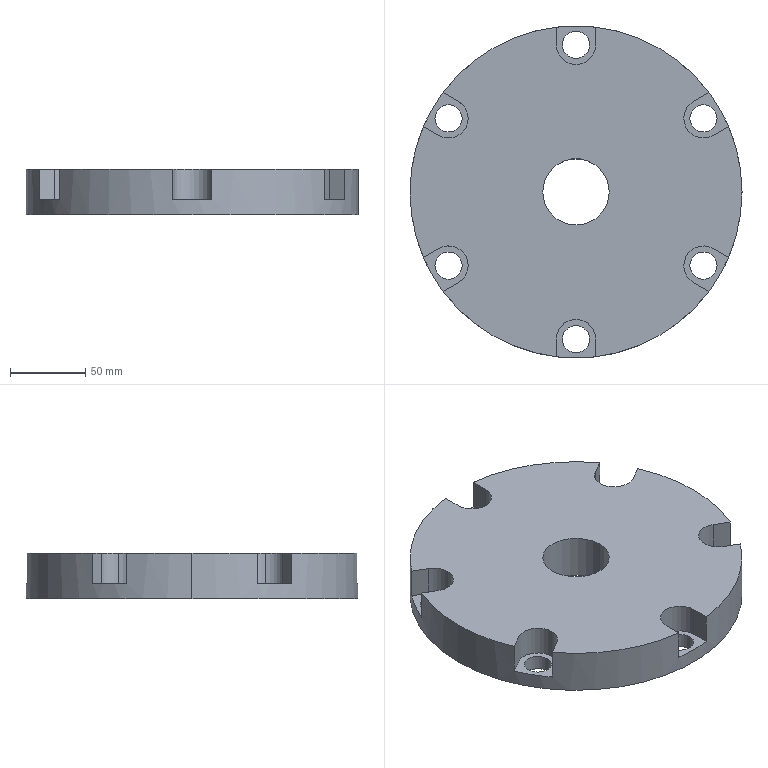Part | SolidWorks | features Extrusion 1, ICE 1 | 1 solid | 44 faces | box 220 x 220 x 30 mm | volume 1009459 mm3 | cylinder 24 | plane 20 | commonest cylinder face diameters 18 x12 26 x8 44 x2 220 x2
STEP:
#1=CARTESIAN_POINT('',(-71.437,-48.75,10.));
#2=VERTEX_POINT('',#1);
#3=CARTESIAN_POINT('',(-90.937,-37.492,10.));
#4=VERTEX_POINT('',#3);
#5=CARTESIAN_POINT('',(-84.437,-48.75,10.));
#6=DIRECTION('',(0.,0.,1.));
#7=DIRECTION('',(1.,0.,0.));
#8=AXIS2_PLACEMENT_3D('',#5,#6,#7);
#9=CIRCLE('',#8,13.);
#10=EDGE_CURVE('',#2,#4,#9,.T.);
#11=ORIENTED_EDGE('',*,*,#10,.F.);
#12=CARTESIAN_POINT('',(-71.437,-48.75,30.));
#13=VERTEX_POINT('',#12);
#14=CARTESIAN_POINT('',(-71.437,-48.75,10.));
#15=DIRECTION('',(0.,0.,1.));
#16=VECTOR('',#15,1000.);
#17=LINE('',#14,#16);
#18=EDGE_CURVE('',#2,#13,#17,.T.);
#19=ORIENTED_EDGE('',*,*,#18,.T.);
#20=CARTESIAN_POINT('',(-90.937,-37.492,30.));
#21=VERTEX_POINT('',#20);
#22=CARTESIAN_POINT('',(-84.437,-48.75,30.));
#23=DIRECTION('',(0.,0.,1.));
#24=DIRECTION('',(1.,0.,0.));
#25=AXIS2_PLACEMENT_3D('',#22,#23,#24);
#26=CIRCLE('',#25,13.);
#27=EDGE_CURVE('',#13,#21,#26,.T.);
#28=ORIENTED_EDGE('',*,*,#27,.T.);
#29=CARTESIAN_POINT('',(-90.937,-37.492,10.));
#30=DIRECTION('',(0.,0.,1.));
#31=VECTOR('',#30,1000.);
#32=LINE('',#29,#31);
#33=EDGE_CURVE('',#4,#21,#32,.T.);
#34=ORIENTED_EDGE('',*,*,#33,.F.);
#35=EDGE_LOOP('',(#11,#19,#28,#34));
#36=FACE_OUTER_BOUND('',#35,.T.);
#37=CARTESIAN_POINT('',(-84.437,-48.75,10.));
#38=DIRECTION('',(0.,0.,1.));
#39=DIRECTION('',(1.,0.,0.));
#40=AXIS2_PLACEMENT_3D('',#37,#38,#39);
#41=CYLINDRICAL_SURFACE('',#40,13.);
#42=ADVANCED_FACE('',(#36),#41,.F.);
#43=CARTESIAN_POINT('',(-71.437,48.75,10.));
#44=VERTEX_POINT('',#43);
#45=CARTESIAN_POINT('',(-77.937,60.008,10.));
#46=VERTEX_POINT('',#45);
#47=CARTESIAN_POINT('',(-84.437,48.75,10.));
#48=DIRECTION('',(0.,0.,1.));
#49=DIRECTION('',(1.,0.,0.));
#50=AXIS2_PLACEMENT_3D('',#47,#48,#49);
#51=CIRCLE('',#50,13.);
#52=EDGE_CURVE('',#44,#46,#51,.T.);
#53=ORIENTED_EDGE('',*,*,#52,.F.);
#54=CARTESIAN_POINT('',(-71.437,48.75,30.));
#55=VERTEX_POINT('',#54);
#56=CARTESIAN_POINT('',(-71.437,48.75,10.));
#57=DIRECTION('',(0.,0.,1.));
#58=VECTOR('',#57,1000.);
#59=LINE('',#56,#58);
#60=EDGE_CURVE('',#44,#55,#59,.T.);
#61=ORIENTED_EDGE('',*,*,#60,.T.);
#62=CARTESIAN_POINT('',(-77.937,60.008,30.));
#63=VERTEX_POINT('',#62);
#64=CARTESIAN_POINT('',(-84.437,48.75,30.));
#65=DIRECTION('',(0.,0.,1.));
#66=DIRECTION('',(1.,0.,0.));
#67=AXIS2_PLACEMENT_3D('',#64,#65,#66);
#68=CIRCLE('',#67,13.);
#69=EDGE_CURVE('',#55,#63,#68,.T.);
#70=ORIENTED_EDGE('',*,*,#69,.T.);
#71=CARTESIAN_POINT('',(-77.937,60.008,10.));
#72=DIRECTION('',(0.,0.,1.));
#73=VECTOR('',#72,1000.);
#74=LINE('',#71,#73);
#75=EDGE_CURVE('',#46,#63,#74,.T.);
#76=ORIENTED_EDGE('',*,*,#75,.F.);
#77=EDGE_LOOP('',(#53,#61,#70,#76));
#78=FACE_OUTER_BOUND('',#77,.T.);
#79=CARTESIAN_POINT('',(-84.437,48.75,10.));
#80=DIRECTION('',(0.,0.,1.));
#81=DIRECTION('',(1.,0.,0.));
#82=AXIS2_PLACEMENT_3D('',#79,#80,#81);
#83=CYLINDRICAL_SURFACE('',#82,13.);
#84=ADVANCED_FACE('',(#78),#83,.F.);
#85=CARTESIAN_POINT('',(-22.,0.,30.));
#86=VERTEX_POINT('',#85);
#87=CARTESIAN_POINT('',(22.,0.,30.));
#88=VERTEX_POINT('',#87);
#89=CARTESIAN_POINT('',(0.,0.,30.));
#90=DIRECTION('',(0.,0.,1.));
#91=DIRECTION('',(1.,0.,0.));
#92=AXIS2_PLACEMENT_3D('',#89,#90,#91);
#93=CIRCLE('',#92,22.);
#94=EDGE_CURVE('',#86,#88,#93,.T.);
#95=ORIENTED_EDGE('',*,*,#94,.T.);
#96=CARTESIAN_POINT('',(22.,0.,0.));
#97=VERTEX_POINT('',#96);
#98=CARTESIAN_POINT('',(22.,0.,30.));
#99=DIRECTION('',(0.,0.,-1.));
#100=VECTOR('',#99,1000.);
#101=LINE('',#98,#100);
#102=EDGE_CURVE('',#88,#97,#101,.T.);
#103=ORIENTED_EDGE('',*,*,#102,.T.);
#104=CARTESIAN_POINT('',(-22.,0.,0.));
#105=VERTEX_POINT('',#104);
#106=CARTESIAN_POINT('',(0.,0.,0.));
#107=DIRECTION('',(0.,0.,1.));
#108=DIRECTION('',(1.,0.,0.));
#109=AXIS2_PLACEMENT_3D('',#106,#107,#108);
#110=CIRCLE('',#109,22.);
#111=EDGE_CURVE('',#105,#97,#110,.T.);
#112=ORIENTED_EDGE('',*,*,#111,.F.);
#113=CARTESIAN_POINT('',(-22.,0.,30.));
#114=DIRECTION('',(0.,0.,-1.));
#115=VECTOR('',#114,1000.);
#116=LINE('',#113,#115);
#117=EDGE_CURVE('',#86,#105,#116,.T.);
#118=ORIENTED_EDGE('',*,*,#117,.F.);
#119=EDGE_LOOP('',(#95,#103,#112,#118));
#120=FACE_OUTER_BOUND('',#119,.T.);
#121=CARTESIAN_POINT('',(0.,0.,30.));
#122=DIRECTION('',(0.,0.,-1.));
#123=DIRECTION('',(-1.,0.,0.));
#124=AXIS2_PLACEMENT_3D('',#121,#122,#123);
#125=CYLINDRICAL_SURFACE('',#124,22.);
#126=ADVANCED_FACE('',(#120),#125,.F.);
#127=CARTESIAN_POINT('',(110.,0.,30.));
#128=VERTEX_POINT('',#127);
#129=CARTESIAN_POINT('',(101.095,43.356,30.));
#130=VERTEX_POINT('',#129);
#131=CARTESIAN_POINT('',(0.,0.,30.));
#132=DIRECTION('',(0.,0.,1.));
#133=DIRECTION('',(1.,0.,0.));
#134=AXIS2_PLACEMENT_3D('',#131,#132,#133);
#135=CIRCLE('',#134,110.);
#136=EDGE_CURVE('',#128,#130,#135,.T.);
#137=ORIENTED_EDGE('',*,*,#136,.F.);
#138=CARTESIAN_POINT('',(110.,0.,0.));
#139=VERTEX_POINT('',#138);
#140=CARTESIAN_POINT('',(110.,0.,30.));
#141=DIRECTION('',(0.,0.,-1.));
#142=VECTOR('',#141,1000.);
#143=LINE('',#140,#142);
#144=EDGE_CURVE('',#128,#139,#143,.T.);
#145=ORIENTED_EDGE('',*,*,#144,.T.);
#146=CARTESIAN_POINT('',(-110.,0.,0.));
#147=VERTEX_POINT('',#146);
#148=CARTESIAN_POINT('',(0.,0.,0.));
#149=DIRECTION('',(0.,0.,1.));
#150=DIRECTION('',(1.,0.,0.));
#151=AXIS2_PLACEMENT_3D('',#148,#149,#150);
#152=CIRCLE('',#151,110.);
#153=EDGE_CURVE('',#139,#147,#152,.T.);
#154=ORIENTED_EDGE('',*,*,#153,.T.);
#155=CARTESIAN_POINT('',(-110.,0.,30.));
#156=VERTEX_POINT('',#155);
#157=CARTESIAN_POINT('',(-110.,0.,30.));
#158=DIRECTION('',(0.,0.,-1.));
#159=VECTOR('',#158,1000.);
#160=LINE('',#157,#159);
#161=EDGE_CURVE('',#156,#147,#160,.T.);
#162=ORIENTED_EDGE('',*,*,#161,.F.);
#163=CARTESIAN_POINT('',(-101.095,43.356,30.));
#164=VERTEX_POINT('',#163);
#165=CARTESIAN_POINT('',(0.,0.,30.));
#166=DIRECTION('',(0.,0.,1.));
#167=DIRECTION('',(1.,0.,0.));
#168=AXIS2_PLACEMENT_3D('',#165,#166,#167);
#169=CIRCLE('',#168,110.);
#170=EDGE_CURVE('',#164,#156,#169,.T.);
#171=ORIENTED_EDGE('',*,*,#170,.F.);
#172=CARTESIAN_POINT('',(-101.095,43.356,10.));
#173=VERTEX_POINT('',#172);
#174=CARTESIAN_POINT('',(-101.095,43.356,30.));
#175=DIRECTION('',(0.,0.,-1.));
#176=VECTOR('',#175,1000.);
#177=LINE('',#174,#176);
#178=EDGE_CURVE('',#164,#173,#177,.T.);
#179=ORIENTED_EDGE('',*,*,#178,.T.);
#180=CARTESIAN_POINT('',(-88.095,65.873,10.));
#181=VERTEX_POINT('',#180);
#182=CARTESIAN_POINT('',(0.,0.,10.));
#183=DIRECTION('',(0.,0.,1.));
#184=DIRECTION('',(1.,0.,0.));
#185=AXIS2_PLACEMENT_3D('',#182,#183,#184);
#186=CIRCLE('',#185,110.);
#187=EDGE_CURVE('',#181,#173,#186,.T.);
#188=ORIENTED_EDGE('',*,*,#187,.F.);
#189=CARTESIAN_POINT('',(-88.095,65.873,30.));
#190=VERTEX_POINT('',#189);
#191=CARTESIAN_POINT('',(-88.095,65.873,30.));
#192=DIRECTION('',(0.,0.,1.));
#193=VECTOR('',#192,1000.);
#194=LINE('',#191,#193);
#195=EDGE_CURVE('',#181,#190,#194,.T.);
#196=ORIENTED_EDGE('',*,*,#195,.T.);
#197=CARTESIAN_POINT('',(-13.,109.229,30.));
#198=VERTEX_POINT('',#197);
#199=CARTESIAN_POINT('',(0.,0.,30.));
#200=DIRECTION('',(0.,0.,1.));
#201=DIRECTION('',(1.,0.,0.));
#202=AXIS2_PLACEMENT_3D('',#199,#200,#201);
#203=CIRCLE('',#202,110.);
#204=EDGE_CURVE('',#198,#190,#203,.T.);
#205=ORIENTED_EDGE('',*,*,#204,.F.);
#206=CARTESIAN_POINT('',(-13.,109.229,10.));
#207=VERTEX_POINT('',#206);
#208=CARTESIAN_POINT('',(-13.,109.229,30.));
#209=DIRECTION('',(0.,0.,-1.));
#210=VECTOR('',#209,1000.);
#211=LINE('',#208,#210);
#212=EDGE_CURVE('',#198,#207,#211,.T.);
#213=ORIENTED_EDGE('',*,*,#212,.T.);
#214=CARTESIAN_POINT('',(13.,109.229,10.));
#215=VERTEX_POINT('',#214);
#216=CARTESIAN_POINT('',(0.,0.,10.));
#217=DIRECTION('',(0.,0.,1.));
#218=DIRECTION('',(1.,0.,0.));
#219=AXIS2_PLACEMENT_3D('',#216,#217,#218);
#220=CIRCLE('',#219,110.);
#221=EDGE_CURVE('',#215,#207,#220,.T.);
#222=ORIENTED_EDGE('',*,*,#221,.F.);
#223=CARTESIAN_POINT('',(13.,109.229,30.));
#224=VERTEX_POINT('',#223);
#225=CARTESIAN_POINT('',(13.,109.229,30.));
#226=DIRECTION('',(0.,0.,1.));
#227=VECTOR('',#226,1000.);
#228=LINE('',#225,#227);
#229=EDGE_CURVE('',#215,#224,#228,.T.);
#230=ORIENTED_EDGE('',*,*,#229,.T.);
#231=CARTESIAN_POINT('',(88.095,65.873,30.));
#232=VERTEX_POINT('',#231);
#233=CARTESIAN_POINT('',(0.,0.,30.));
#234=DIRECTION('',(0.,0.,1.));
#235=DIRECTION('',(1.,0.,0.));
#236=AXIS2_PLACEMENT_3D('',#233,#234,#235);
#237=CIRCLE('',#236,110.);
#238=EDGE_CURVE('',#232,#224,#237,.T.);
#239=ORIENTED_EDGE('',*,*,#238,.F.);
#240=CARTESIAN_POINT('',(88.095,65.873,10.));
#241=VERTEX_POINT('',#240);
#242=CARTESIAN_POINT('',(88.095,65.873,30.));
#243=DIRECTION('',(0.,0.,-1.));
#244=VECTOR('',#243,1000.);
#245=LINE('',#242,#244);
#246=EDGE_CURVE('',#232,#241,#245,.T.);
#247=ORIENTED_EDGE('',*,*,#246,.T.);
#248=CARTESIAN_POINT('',(101.095,43.356,10.));
#249=VERTEX_POINT('',#248);
#250=CARTESIAN_POINT('',(0.,0.,10.));
#251=DIRECTION('',(0.,0.,1.));
#252=DIRECTION('',(1.,0.,0.));
#253=AXIS2_PLACEMENT_3D('',#250,#251,#252);
#254=CIRCLE('',#253,110.);
#255=EDGE_CURVE('',#249,#241,#254,.T.);
#256=ORIENTED_EDGE('',*,*,#255,.F.);
#257=CARTESIAN_POINT('',(101.095,43.356,30.));
#258=DIRECTION('',(0.,0.,1.));
#259=VECTOR('',#258,1000.);
#260=LINE('',#257,#259);
#261=EDGE_CURVE('',#249,#130,#260,.T.);
#262=ORIENTED_EDGE('',*,*,#261,.T.);
#263=EDGE_LOOP('',(#137,#145,#154,#162,#171,#179,#188,#196,#205,#213,#222,#230,#239,#247,#256,#262));
#264=FACE_OUTER_BOUND('',#263,.T.);
#265=CARTESIAN_POINT('',(0.,0.,30.));
#266=DIRECTION('',(0.,0.,-1.));
#267=DIRECTION('',(-1.,0.,0.));
#268=AXIS2_PLACEMENT_3D('',#265,#266,#267);
#269=CYLINDRICAL_SURFACE('',#268,110.);
#270=ADVANCED_FACE('',(#264),#269,.T.);
#271=CARTESIAN_POINT('',(-93.437,48.75,10.));
#272=VERTEX_POINT('',#271);
#273=CARTESIAN_POINT('',(-75.437,48.75,10.));
#274=VERTEX_POINT('',#273);
#275=CARTESIAN_POINT('',(-84.437,48.75,10.));
#276=DIRECTION('',(0.,0.,1.));
#277=DIRECTION('',(1.,0.,0.));
#278=AXIS2_PLACEMENT_3D('',#275,#276,#277);
#279=CIRCLE('',#278,9.);
#280=EDGE_CURVE('',#272,#274,#279,.T.);
#281=ORIENTED_EDGE('',*,*,#280,.T.);
#282=CARTESIAN_POINT('',(-75.437,48.75,0.));
#283=VERTEX_POINT('',#282);
#284=CARTESIAN_POINT('',(-75.437,48.75,30.));
#285=DIRECTION('',(0.,0.,-1.));
#286=VECTOR('',#285,1000.);
#287=LINE('',#284,#286);
#288=EDGE_CURVE('',#274,#283,#287,.T.);
#289=ORIENTED_EDGE('',*,*,#288,.T.);
#290=CARTESIAN_POINT('',(-93.437,48.75,0.));
#291=VERTEX_POINT('',#290);
#292=CARTESIAN_POINT('',(-84.437,48.75,0.));
#293=DIRECTION('',(0.,0.,1.));
#294=DIRECTION('',(1.,0.,0.));
#295=AXIS2_PLACEMENT_3D('',#292,#293,#294);
#296=CIRCLE('',#295,9.);
#297=EDGE_CURVE('',#291,#283,#296,.T.);
#298=ORIENTED_EDGE('',*,*,#297,.F.);
#299=CARTESIAN_POINT('',(-93.437,48.75,30.));
#300=DIRECTION('',(0.,0.,-1.));
#301=VECTOR('',#300,1000.);
#302=LINE('',#299,#301);
#303=EDGE_CURVE('',#272,#291,#302,.T.);
#304=ORIENTED_EDGE('',*,*,#303,.F.);
#305=EDGE_LOOP('',(#281,#289,#298,#304));
#306=FACE_OUTER_BOUND('',#305,.T.);
#307=CARTESIAN_POINT('',(-84.437,48.75,30.));
#308=DIRECTION('',(0.,0.,-1.));
#309=DIRECTION('',(-1.,0.,0.));
#310=AXIS2_PLACEMENT_3D('',#307,#308,#309);
#311=CYLINDRICAL_SURFACE('',#310,9.);
#312=ADVANCED_FACE('',(#306),#311,.F.);
#313=CARTESIAN_POINT('',(-93.437,-48.75,10.));
#314=VERTEX_POINT('',#313);
#315=CARTESIAN_POINT('',(-75.437,-48.75,10.));
#316=VERTEX_POINT('',#315);
#317=CARTESIAN_POINT('',(-84.437,-48.75,10.));
#318=DIRECTION('',(0.,0.,1.));
#319=DIRECTION('',(1.,0.,0.));
#320=AXIS2_PLACEMENT_3D('',#317,#318,#319);
#321=CIRCLE('',#320,9.);
#322=EDGE_CURVE('',#314,#316,#321,.T.);
#323=ORIENTED_EDGE('',*,*,#322,.T.);
#324=CARTESIAN_POINT('',(-75.437,-48.75,0.));
#325=VERTEX_POINT('',#324);
#326=CARTESIAN_POINT('',(-75.437,-48.75,30.));
#327=DIRECTION('',(0.,0.,-1.));
#328=VECTOR('',#327,1000.);
#329=LINE('',#326,#328);
#330=EDGE_CURVE('',#316,#325,#329,.T.);
#331=ORIENTED_EDGE('',*,*,#330,.T.);
#332=CARTESIAN_POINT('',(-93.437,-48.75,0.));
#333=VERTEX_POINT('',#332);
#334=CARTESIAN_POINT('',(-84.437,-48.75,0.));
#335=DIRECTION('',(0.,0.,1.));
#336=DIRECTION('',(1.,0.,0.));
#337=AXIS2_PLACEMENT_3D('',#334,#335,#336);
#338=CIRCLE('',#337,9.);
#339=EDGE_CURVE('',#333,#325,#338,.T.);
#340=ORIENTED_EDGE('',*,*,#339,.F.);
#341=CARTESIAN_POINT('',(-93.437,-48.75,30.));
#342=DIRECTION('',(0.,0.,-1.));
#343=VECTOR('',#342,1000.);
#344=LINE('',#341,#343);
#345=EDGE_CURVE('',#314,#333,#344,.T.);
#346=ORIENTED_EDGE('',*,*,#345,.F.);
#347=EDGE_LOOP('',(#323,#331,#340,#346));
#348=FACE_OUTER_BOUND('',#347,.T.);
#349=CARTESIAN_POINT('',(-84.437,-48.75,30.));
#350=DIRECTION('',(0.,0.,-1.));
#351=DIRECTION('',(-1.,0.,0.));
#352=AXIS2_PLACEMENT_3D('',#349,#350,#351);
#353=CYLINDRICAL_SURFACE('',#352,9.);
#354=ADVANCED_FACE('',(#348),#353,.F.);
#355=CARTESIAN_POINT('',(-9.,-97.5,10.));
#356=VERTEX_POINT('',#355);
#357=CARTESIAN_POINT('',(9.,-97.5,10.));
#358=VERTEX_POINT('',#357);
#359=CARTESIAN_POINT('',(0.,-97.5,10.));
#360=DIRECTION('',(0.,0.,1.));
#361=DIRECTION('',(1.,0.,0.));
#362=AXIS2_PLACEMENT_3D('',#359,#360,#361);
#363=CIRCLE('',#362,9.);
#364=EDGE_CURVE('',#356,#358,#363,.T.);
#365=ORIENTED_EDGE('',*,*,#364,.T.);
#366=CARTESIAN_POINT('',(9.,-97.5,0.));
#367=VERTEX_POINT('',#366);
#368=CARTESIAN_POINT('',(9.,-97.5,30.));
#369=DIRECTION('',(0.,0.,-1.));
#370=VECTOR('',#369,1000.);
#371=LINE('',#368,#370);
#372=EDGE_CURVE('',#358,#367,#371,.T.);
#373=ORIENTED_EDGE('',*,*,#372,.T.);
#374=CARTESIAN_POINT('',(-9.,-97.5,0.));
#375=VERTEX_POINT('',#374);
#376=CARTESIAN_POINT('',(0.,-97.5,0.));
#377=DIRECTION('',(0.,0.,1.));
#378=DIRECTION('',(1.,0.,0.));
#379=AXIS2_PLACEMENT_3D('',#376,#377,#378);
#380=CIRCLE('',#379,9.);
#381=EDGE_CURVE('',#375,#367,#380,.T.);
#382=ORIENTED_EDGE('',*,*,#381,.F.);
#383=CARTESIAN_POINT('',(-9.,-97.5,30.));
#384=DIRECTION('',(0.,0.,-1.));
#385=VECTOR('',#384,1000.);
#386=LINE('',#383,#385);
#387=EDGE_CURVE('',#356,#375,#386,.T.);
#388=ORIENTED_EDGE('',*,*,#387,.F.);
#389=EDGE_LOOP('',(#365,#373,#382,#388));
#390=FACE_OUTER_BOUND('',#389,.T.);
#391=CARTESIAN_POINT('',(0.,-97.5,30.));
#392=DIRECTION('',(0.,0.,-1.));
#393=DIRECTION('',(-1.,0.,0.));
#394=AXIS2_PLACEMENT_3D('',#391,#392,#393);
#395=CYLINDRICAL_SURFACE('',#394,9.);
#396=ADVANCED_FACE('',(#390),#395,.F.);
#397=CARTESIAN_POINT('',(75.437,-48.75,10.));
#398=VERTEX_POINT('',#397);
#399=CARTESIAN_POINT('',(93.437,-48.75,10.));
#400=VERTEX_POINT('',#399);
#401=CARTESIAN_POINT('',(84.437,-48.75,10.));
#402=DIRECTION('',(0.,0.,1.));
#403=DIRECTION('',(1.,0.,0.));
#404=AXIS2_PLACEMENT_3D('',#401,#402,#403);
#405=CIRCLE('',#404,9.);
#406=EDGE_CURVE('',#398,#400,#405,.T.);
#407=ORIENTED_EDGE('',*,*,#406,.T.);
#408=CARTESIAN_POINT('',(93.437,-48.75,0.));
#409=VERTEX_POINT('',#408);
#410=CARTESIAN_POINT('',(93.437,-48.75,30.));
#411=DIRECTION('',(0.,0.,-1.));
#412=VECTOR('',#411,1000.);
#413=LINE('',#410,#412);
#414=EDGE_CURVE('',#400,#409,#413,.T.);
#415=ORIENTED_EDGE('',*,*,#414,.T.);
#416=CARTESIAN_POINT('',(75.437,-48.75,0.));
#417=VERTEX_POINT('',#416);
#418=CARTESIAN_POINT('',(84.437,-48.75,0.));
#419=DIRECTION('',(0.,0.,1.));
#420=DIRECTION('',(1.,0.,0.));
#421=AXIS2_PLACEMENT_3D('',#418,#419,#420);
#422=CIRCLE('',#421,9.);
#423=EDGE_CURVE('',#417,#409,#422,.T.);
#424=ORIENTED_EDGE('',*,*,#423,.F.);
#425=CARTESIAN_POINT('',(75.437,-48.75,30.));
#426=DIRECTION('',(0.,0.,-1.));
#427=VECTOR('',#426,1000.);
#428=LINE('',#425,#427);
#429=EDGE_CURVE('',#398,#417,#428,.T.);
#430=ORIENTED_EDGE('',*,*,#429,.F.);
#431=EDGE_LOOP('',(#407,#415,#424,#430));
#432=FACE_OUTER_BOUND('',#431,.T.);
#433=CARTESIAN_POINT('',(84.437,-48.75,30.));
#434=DIRECTION('',(0.,0.,-1.));
#435=DIRECTION('',(-1.,0.,0.));
#436=AXIS2_PLACEMENT_3D('',#433,#434,#435);
#437=CYLINDRICAL_SURFACE('',#436,9.);
#438=ADVANCED_FACE('',(#432),#437,.F.);
#439=CARTESIAN_POINT('',(75.437,48.75,10.));
#440=VERTEX_POINT('',#439);
#441=CARTESIAN_POINT('',(93.437,48.75,10.));
#442=VERTEX_POINT('',#441);
#443=CARTESIAN_POINT('',(84.437,48.75,10.));
#444=DIRECTION('',(0.,0.,1.));
#445=DIRECTION('',(1.,0.,0.));
#446=AXIS2_PLACEMENT_3D('',#443,#444,#445);
#447=CIRCLE('',#446,9.);
#448=EDGE_CURVE('',#440,#442,#447,.T.);
#449=ORIENTED_EDGE('',*,*,#448,.T.);
#450=CARTESIAN_POINT('',(93.437,48.75,0.));
#451=VERTEX_POINT('',#450);
#452=CARTESIAN_POINT('',(93.437,48.75,30.));
#453=DIRECTION('',(0.,0.,-1.));
#454=VECTOR('',#453,1000.);
#455=LINE('',#452,#454);
#456=EDGE_CURVE('',#442,#451,#455,.T.);
#457=ORIENTED_EDGE('',*,*,#456,.T.);
#458=CARTESIAN_POINT('',(75.437,48.75,0.));
#459=VERTEX_POINT('',#458);
#460=CARTESIAN_POINT('',(84.437,48.75,0.));
#461=DIRECTION('',(0.,0.,1.));
#462=DIRECTION('',(1.,0.,0.));
#463=AXIS2_PLACEMENT_3D('',#460,#461,#462);
#464=CIRCLE('',#463,9.);
#465=EDGE_CURVE('',#459,#451,#464,.T.);
#466=ORIENTED_EDGE('',*,*,#465,.F.);
#467=CARTESIAN_POINT('',(75.437,48.75,30.));
#468=DIRECTION('',(0.,0.,-1.));
#469=VECTOR('',#468,1000.);
#470=LINE('',#467,#469);
#471=EDGE_CURVE('',#440,#459,#470,.T.);
#472=ORIENTED_EDGE('',*,*,#471,.F.);
#473=EDGE_LOOP('',(#449,#457,#466,#472));
#474=FACE_OUTER_BOUND('',#473,.T.);
#475=CARTESIAN_POINT('',(84.437,48.75,30.));
#476=DIRECTION('',(0.,0.,-1.));
#477=DIRECTION('',(-1.,0.,0.));
#478=AXIS2_PLACEMENT_3D('',#475,#476,#477);
#479=CYLINDRICAL_SURFACE('',#478,9.);
#480=ADVANCED_FACE('',(#474),#479,.F.);
#481=CARTESIAN_POINT('',(-9.,97.5,10.));
#482=VERTEX_POINT('',#481);
#483=CARTESIAN_POINT('',(9.,97.5,10.));
#484=VERTEX_POINT('',#483);
#485=CARTESIAN_POINT('',(0.,97.5,10.));
#486=DIRECTION('',(0.,0.,1.));
#487=DIRECTION('',(1.,0.,0.));
#488=AXIS2_PLACEMENT_3D('',#485,#486,#487);
#489=CIRCLE('',#488,9.);
#490=EDGE_CURVE('',#482,#484,#489,.T.);
#491=ORIENTED_EDGE('',*,*,#490,.T.);
#492=CARTESIAN_POINT('',(9.,97.5,0.));
#493=VERTEX_POINT('',#492);
#494=CARTESIAN_POINT('',(9.,97.5,30.));
#495=DIRECTION('',(0.,0.,-1.));
#496=VECTOR('',#495,1000.);
#497=LINE('',#494,#496);
#498=EDGE_CURVE('',#484,#493,#497,.T.);
#499=ORIENTED_EDGE('',*,*,#498,.T.);
#500=CARTESIAN_POINT('',(-9.,97.5,0.));
#501=VERTEX_POINT('',#500);
#502=CARTESIAN_POINT('',(0.,97.5,0.));
#503=DIRECTION('',(0.,0.,1.));
#504=DIRECTION('',(1.,0.,0.));
#505=AXIS2_PLACEMENT_3D('',#502,#503,#504);
#506=CIRCLE('',#505,9.);
#507=EDGE_CURVE('',#501,#493,#506,.T.);
#508=ORIENTED_EDGE('',*,*,#507,.F.);
#509=CARTESIAN_POINT('',(-9.,97.5,30.));
#510=DIRECTION('',(0.,0.,-1.));
#511=VECTOR('',#510,1000.);
#512=LINE('',#509,#511);
#513=EDGE_CURVE('',#482,#501,#512,.T.);
#514=ORIENTED_EDGE('',*,*,#513,.F.);
#515=EDGE_LOOP('',(#491,#499,#508,#514));
#516=FACE_OUTER_BOUND('',#515,.T.);
#517=CARTESIAN_POINT('',(0.,97.5,30.));
#518=DIRECTION('',(0.,0.,-1.));
#519=DIRECTION('',(-1.,0.,0.));
#520=AXIS2_PLACEMENT_3D('',#517,#518,#519);
#521=CYLINDRICAL_SURFACE('',#520,9.);
#522=ADVANCED_FACE('',(#516),#521,.F.);
#523=ORIENTED_EDGE('',*,*,#498,.F.);
#524=CARTESIAN_POINT('',(0.,97.5,10.));
#525=DIRECTION('',(0.,0.,1.));
#526=DIRECTION('',(1.,0.,0.));
#527=AXIS2_PLACEMENT_3D('',#524,#525,#526);
#528=CIRCLE('',#527,9.);
#529=EDGE_CURVE('',#484,#482,#528,.T.);
#530=ORIENTED_EDGE('',*,*,#529,.T.);
#531=ORIENTED_EDGE('',*,*,#513,.T.);
#532=CARTESIAN_POINT('',(0.,97.5,0.));
#533=DIRECTION('',(0.,0.,1.));
#534=DIRECTION('',(1.,0.,0.));
#535=AXIS2_PLACEMENT_3D('',#532,#533,#534);
#536=CIRCLE('',#535,9.);
#537=EDGE_CURVE('',#493,#501,#536,.T.);
#538=ORIENTED_EDGE('',*,*,#537,.F.);
#539=EDGE_LOOP('',(#523,#530,#531,#538));
#540=FACE_OUTER_BOUND('',#539,.T.);
#541=CARTESIAN_POINT('',(0.,97.5,30.));
#542=DIRECTION('',(0.,0.,-1.));
#543=DIRECTION('',(-1.,0.,0.));
#544=AXIS2_PLACEMENT_3D('',#541,#542,#543);
#545=CYLINDRICAL_SURFACE('',#544,9.);
#546=ADVANCED_FACE('',(#540),#545,.F.);
#547=ORIENTED_EDGE('',*,*,#456,.F.);
#548=CARTESIAN_POINT('',(84.437,48.75,10.));
#549=DIRECTION('',(0.,0.,1.));
#550=DIRECTION('',(1.,0.,0.));
#551=AXIS2_PLACEMENT_3D('',#548,#549,#550);
#552=CIRCLE('',#551,9.);
#553=EDGE_CURVE('',#442,#440,#552,.T.);
#554=ORIENTED_EDGE('',*,*,#553,.T.);
#555=ORIENTED_EDGE('',*,*,#471,.T.);
#556=CARTESIAN_POINT('',(84.437,48.75,0.));
#557=DIRECTION('',(0.,0.,1.));
#558=DIRECTION('',(1.,0.,0.));
#559=AXIS2_PLACEMENT_3D('',#556,#557,#558);
#560=CIRCLE('',#559,9.);
#561=EDGE_CURVE('',#451,#459,#560,.T.);
#562=ORIENTED_EDGE('',*,*,#561,.F.);
#563=EDGE_LOOP('',(#547,#554,#555,#562));
#564=FACE_OUTER_BOUND('',#563,.T.);
#565=CARTESIAN_POINT('',(84.437,48.75,30.));
#566=DIRECTION('',(0.,0.,-1.));
#567=DIRECTION('',(-1.,0.,0.));
#568=AXIS2_PLACEMENT_3D('',#565,#566,#567);
#569=CYLINDRICAL_SURFACE('',#568,9.);
#570=ADVANCED_FACE('',(#564),#569,.F.);
#571=ORIENTED_EDGE('',*,*,#414,.F.);
#572=CARTESIAN_POINT('',(84.437,-48.75,10.));
#573=DIRECTION('',(0.,0.,1.));
#574=DIRECTION('',(1.,0.,0.));
#575=AXIS2_PLACEMENT_3D('',#572,#573,#574);
#576=CIRCLE('',#575,9.);
#577=EDGE_CURVE('',#400,#398,#576,.T.);
#578=ORIENTED_EDGE('',*,*,#577,.T.);
#579=ORIENTED_EDGE('',*,*,#429,.T.);
#580=CARTESIAN_POINT('',(84.437,-48.75,0.));
#581=DIRECTION('',(0.,0.,1.));
#582=DIRECTION('',(1.,0.,0.));
#583=AXIS2_PLACEMENT_3D('',#580,#581,#582);
#584=CIRCLE('',#583,9.);
#585=EDGE_CURVE('',#409,#417,#584,.T.);
#586=ORIENTED_EDGE('',*,*,#585,.F.);
#587=EDGE_LOOP('',(#571,#578,#579,#586));
#588=FACE_OUTER_BOUND('',#587,.T.);
#589=CARTESIAN_POINT('',(84.437,-48.75,30.));
#590=DIRECTION('',(0.,0.,-1.));
#591=DIRECTION('',(-1.,0.,0.));
#592=AXIS2_PLACEMENT_3D('',#589,#590,#591);
#593=CYLINDRICAL_SURFACE('',#592,9.);
#594=ADVANCED_FACE('',(#588),#593,.F.);
#595=ORIENTED_EDGE('',*,*,#372,.F.);
#596=CARTESIAN_POINT('',(0.,-97.5,10.));
#597=DIRECTION('',(0.,0.,1.));
#598=DIRECTION('',(1.,0.,0.));
#599=AXIS2_PLACEMENT_3D('',#596,#597,#598);
#600=CIRCLE('',#599,9.);
#601=EDGE_CURVE('',#358,#356,#600,.T.);
#602=ORIENTED_EDGE('',*,*,#601,.T.);
#603=ORIENTED_EDGE('',*,*,#387,.T.);
#604=CARTESIAN_POINT('',(0.,-97.5,0.));
#605=DIRECTION('',(0.,0.,1.));
#606=DIRECTION('',(1.,0.,0.));
#607=AXIS2_PLACEMENT_3D('',#604,#605,#606);
#608=CIRCLE('',#607,9.);
#609=EDGE_CURVE('',#367,#375,#608,.T.);
#610=ORIENTED_EDGE('',*,*,#609,.F.);
#611=EDGE_LOOP('',(#595,#602,#603,#610));
#612=FACE_OUTER_BOUND('',#611,.T.);
#613=CARTESIAN_POINT('',(0.,-97.5,30.));
#614=DIRECTION('',(0.,0.,-1.));
#615=DIRECTION('',(-1.,0.,0.));
#616=AXIS2_PLACEMENT_3D('',#613,#614,#615);
#617=CYLINDRICAL_SURFACE('',#616,9.);
#618=ADVANCED_FACE('',(#612),#617,.F.);
#619=ORIENTED_EDGE('',*,*,#330,.F.);
#620=CARTESIAN_POINT('',(-84.437,-48.75,10.));
#621=DIRECTION('',(0.,0.,1.));
#622=DIRECTION('',(1.,0.,0.));
#623=AXIS2_PLACEMENT_3D('',#620,#621,#622);
#624=CIRCLE('',#623,9.);
#625=EDGE_CURVE('',#316,#314,#624,.T.);
#626=ORIENTED_EDGE('',*,*,#625,.T.);
#627=ORIENTED_EDGE('',*,*,#345,.T.);
#628=CARTESIAN_POINT('',(-84.437,-48.75,0.));
#629=DIRECTION('',(0.,0.,1.));
#630=DIRECTION('',(1.,0.,0.));
#631=AXIS2_PLACEMENT_3D('',#628,#629,#630);
#632=CIRCLE('',#631,9.);
#633=EDGE_CURVE('',#325,#333,#632,.T.);
#634=ORIENTED_EDGE('',*,*,#633,.F.);
#635=EDGE_LOOP('',(#619,#626,#627,#634));
#636=FACE_OUTER_BOUND('',#635,.T.);
#637=CARTESIAN_POINT('',(-84.437,-48.75,30.));
#638=DIRECTION('',(0.,0.,-1.));
#639=DIRECTION('',(-1.,0.,0.));
#640=AXIS2_PLACEMENT_3D('',#637,#638,#639);
#641=CYLINDRICAL_SURFACE('',#640,9.);
#642=ADVANCED_FACE('',(#636),#641,.F.);
#643=ORIENTED_EDGE('',*,*,#288,.F.);
#644=CARTESIAN_POINT('',(-84.437,48.75,10.));
#645=DIRECTION('',(0.,0.,1.));
#646=DIRECTION('',(1.,0.,0.));
#647=AXIS2_PLACEMENT_3D('',#644,#645,#646);
#648=CIRCLE('',#647,9.);
#649=EDGE_CURVE('',#274,#272,#648,.T.);
#650=ORIENTED_EDGE('',*,*,#649,.T.);
#651=ORIENTED_EDGE('',*,*,#303,.T.);
#652=CARTESIAN_POINT('',(-84.437,48.75,0.));
#653=DIRECTION('',(0.,0.,1.));
#654=DIRECTION('',(1.,0.,0.));
#655=AXIS2_PLACEMENT_3D('',#652,#653,#654);
#656=CIRCLE('',#655,9.);
#657=EDGE_CURVE('',#283,#291,#656,.T.);
#658=ORIENTED_EDGE('',*,*,#657,.F.);
#659=EDGE_LOOP('',(#643,#650,#651,#658));
#660=FACE_OUTER_BOUND('',#659,.T.);
#661=CARTESIAN_POINT('',(-84.437,48.75,30.));
#662=DIRECTION('',(0.,0.,-1.));
#663=DIRECTION('',(-1.,0.,0.));
#664=AXIS2_PLACEMENT_3D('',#661,#662,#663);
#665=CYLINDRICAL_SURFACE('',#664,9.);
#666=ADVANCED_FACE('',(#660),#665,.F.);
#667=CARTESIAN_POINT('',(-13.,97.5,30.));
#668=VERTEX_POINT('',#667);
#669=CARTESIAN_POINT('',(-13.,97.5,30.));
#670=DIRECTION('',(0.,-1.,0.));
#671=VECTOR('',#670,1000.);
#672=LINE('',#669,#671);
#673=EDGE_CURVE('',#198,#668,#672,.T.);
#674=ORIENTED_EDGE('',*,*,#673,.F.);
#675=ORIENTED_EDGE('',*,*,#204,.T.);
#676=CARTESIAN_POINT('',(-92.687,68.524,30.));
#677=DIRECTION('',(-0.866,0.5,0.));
#678=VECTOR('',#677,1000.);
#679=LINE('',#676,#678);
#680=EDGE_CURVE('',#63,#190,#679,.T.);
#681=ORIENTED_EDGE('',*,*,#680,.F.);
#682=ORIENTED_EDGE('',*,*,#69,.F.);
#683=CARTESIAN_POINT('',(-90.937,37.492,30.));
#684=VERTEX_POINT('',#683);
#685=CARTESIAN_POINT('',(-84.437,48.75,30.));
#686=DIRECTION('',(0.,0.,1.));
#687=DIRECTION('',(1.,0.,0.));
#688=AXIS2_PLACEMENT_3D('',#685,#686,#687);
#689=CIRCLE('',#688,13.);
#690=EDGE_CURVE('',#684,#55,#689,.T.);
#691=ORIENTED_EDGE('',*,*,#690,.F.);
#692=CARTESIAN_POINT('',(-90.937,37.492,30.));
#693=DIRECTION('',(0.866,-0.5,0.));
#694=VECTOR('',#693,1000.);
#695=LINE('',#692,#694);
#696=EDGE_CURVE('',#164,#684,#695,.T.);
#697=ORIENTED_EDGE('',*,*,#696,.F.);
#698=ORIENTED_EDGE('',*,*,#170,.T.);
#699=CARTESIAN_POINT('',(-101.095,-43.356,30.));
#700=VERTEX_POINT('',#699);
#701=CARTESIAN_POINT('',(0.,0.,30.));
#702=DIRECTION('',(0.,0.,1.));
#703=DIRECTION('',(1.,0.,0.));
#704=AXIS2_PLACEMENT_3D('',#701,#702,#703);
#705=CIRCLE('',#704,110.);
#706=EDGE_CURVE('',#156,#700,#705,.T.);
#707=ORIENTED_EDGE('',*,*,#706,.T.);
#708=CARTESIAN_POINT('',(-105.687,-46.007,30.));
#709=DIRECTION('',(-0.866,-0.5,0.));
#710=VECTOR('',#709,1000.);
#711=LINE('',#708,#710);
#712=EDGE_CURVE('',#21,#700,#711,.T.);
#713=ORIENTED_EDGE('',*,*,#712,.F.);
#714=ORIENTED_EDGE('',*,*,#27,.F.);
#715=CARTESIAN_POINT('',(-77.937,-60.008,30.));
#716=VERTEX_POINT('',#715);
#717=CARTESIAN_POINT('',(-84.437,-48.75,30.));
#718=DIRECTION('',(0.,0.,1.));
#719=DIRECTION('',(1.,0.,0.));
#720=AXIS2_PLACEMENT_3D('',#717,#718,#719);
#721=CIRCLE('',#720,13.);
#722=EDGE_CURVE('',#716,#13,#721,.T.);
#723=ORIENTED_EDGE('',*,*,#722,.F.);
#724=CARTESIAN_POINT('',(-88.095,-65.873,30.));
#725=VERTEX_POINT('',#724);
#726=CARTESIAN_POINT('',(-77.937,-60.008,30.));
#727=DIRECTION('',(0.866,0.5,0.));
#728=VECTOR('',#727,1000.);
#729=LINE('',#726,#728);
#730=EDGE_CURVE('',#725,#716,#729,.T.);
#731=ORIENTED_EDGE('',*,*,#730,.F.);
#732=CARTESIAN_POINT('',(-13.,-109.229,30.));
#733=VERTEX_POINT('',#732);
#734=CARTESIAN_POINT('',(0.,0.,30.));
#735=DIRECTION('',(0.,0.,1.));
#736=DIRECTION('',(1.,0.,0.));
#737=AXIS2_PLACEMENT_3D('',#734,#735,#736);
#738=CIRCLE('',#737,110.);
#739=EDGE_CURVE('',#725,#733,#738,.T.);
#740=ORIENTED_EDGE('',*,*,#739,.T.);
#741=CARTESIAN_POINT('',(-13.,-97.5,30.));
#742=VERTEX_POINT('',#741);
#743=CARTESIAN_POINT('',(-13.,-114.531,30.));
#744=DIRECTION('',(0.,-1.,0.));
#745=VECTOR('',#744,1000.);
#746=LINE('',#743,#745);
#747=EDGE_CURVE('',#742,#733,#746,.T.);
#748=ORIENTED_EDGE('',*,*,#747,.F.);
#749=CARTESIAN_POINT('',(13.,-97.5,30.));
#750=VERTEX_POINT('',#749);
#751=CARTESIAN_POINT('',(0.,-97.5,30.));
#752=DIRECTION('',(0.,0.,1.));
#753=DIRECTION('',(1.,0.,0.));
#754=AXIS2_PLACEMENT_3D('',#751,#752,#753);
#755=CIRCLE('',#754,13.);
#756=EDGE_CURVE('',#750,#742,#755,.T.);
#757=ORIENTED_EDGE('',*,*,#756,.F.);
#758=CARTESIAN_POINT('',(13.,-109.229,30.));
#759=VERTEX_POINT('',#758);
#760=CARTESIAN_POINT('',(13.,-97.5,30.));
#761=DIRECTION('',(0.,1.,0.));
#762=VECTOR('',#761,1000.);
#763=LINE('',#760,#762);
#764=EDGE_CURVE('',#759,#750,#763,.T.);
#765=ORIENTED_EDGE('',*,*,#764,.F.);
#766=CARTESIAN_POINT('',(88.095,-65.873,30.));
#767=VERTEX_POINT('',#766);
#768=CARTESIAN_POINT('',(0.,0.,30.));
#769=DIRECTION('',(0.,0.,1.));
#770=DIRECTION('',(1.,0.,0.));
#771=AXIS2_PLACEMENT_3D('',#768,#769,#770);
#772=CIRCLE('',#771,110.);
#773=EDGE_CURVE('',#759,#767,#772,.T.);
#774=ORIENTED_EDGE('',*,*,#773,.T.);
#775=CARTESIAN_POINT('',(77.937,-60.008,30.));
#776=VERTEX_POINT('',#775);
#777=CARTESIAN_POINT('',(92.687,-68.524,30.));
#778=DIRECTION('',(0.866,-0.5,0.));
#779=VECTOR('',#778,1000.);
#780=LINE('',#777,#779);
#781=EDGE_CURVE('',#776,#767,#780,.T.);
#782=ORIENTED_EDGE('',*,*,#781,.F.);
#783=CARTESIAN_POINT('',(90.937,-37.492,30.));
#784=VERTEX_POINT('',#783);
#785=CARTESIAN_POINT('',(84.437,-48.75,30.));
#786=DIRECTION('',(0.,0.,1.));
#787=DIRECTION('',(1.,0.,0.));
#788=AXIS2_PLACEMENT_3D('',#785,#786,#787);
#789=CIRCLE('',#788,13.);
#790=EDGE_CURVE('',#784,#776,#789,.T.);
#791=ORIENTED_EDGE('',*,*,#790,.F.);
#792=CARTESIAN_POINT('',(101.095,-43.356,30.));
#793=VERTEX_POINT('',#792);
#794=CARTESIAN_POINT('',(90.937,-37.492,30.));
#795=DIRECTION('',(-0.866,0.5,0.));
#796=VECTOR('',#795,1000.);
#797=LINE('',#794,#796);
#798=EDGE_CURVE('',#793,#784,#797,.T.);
#799=ORIENTED_EDGE('',*,*,#798,.F.);
#800=CARTESIAN_POINT('',(0.,0.,30.));
#801=DIRECTION('',(0.,0.,1.));
#802=DIRECTION('',(1.,0.,0.));
#803=AXIS2_PLACEMENT_3D('',#800,#801,#802);
#804=CIRCLE('',#803,110.);
#805=EDGE_CURVE('',#793,#128,#804,.T.);
#806=ORIENTED_EDGE('',*,*,#805,.T.);
#807=ORIENTED_EDGE('',*,*,#136,.T.);
#808=CARTESIAN_POINT('',(90.937,37.492,30.));
#809=VERTEX_POINT('',#808);
#810=CARTESIAN_POINT('',(105.687,46.007,30.));
#811=DIRECTION('',(0.866,0.5,0.));
#812=VECTOR('',#811,1000.);
#813=LINE('',#810,#812);
#814=EDGE_CURVE('',#809,#130,#813,.T.);
#815=ORIENTED_EDGE('',*,*,#814,.F.);
#816=CARTESIAN_POINT('',(77.937,60.008,30.));
#817=VERTEX_POINT('',#816);
#818=CARTESIAN_POINT('',(84.437,48.75,30.));
#819=DIRECTION('',(0.,0.,1.));
#820=DIRECTION('',(1.,0.,0.));
#821=AXIS2_PLACEMENT_3D('',#818,#819,#820);
#822=CIRCLE('',#821,13.);
#823=EDGE_CURVE('',#817,#809,#822,.T.);
#824=ORIENTED_EDGE('',*,*,#823,.F.);
#825=CARTESIAN_POINT('',(77.937,60.008,30.));
#826=DIRECTION('',(-0.866,-0.5,0.));
#827=VECTOR('',#826,1000.);
#828=LINE('',#825,#827);
#829=EDGE_CURVE('',#232,#817,#828,.T.);
#830=ORIENTED_EDGE('',*,*,#829,.F.);
#831=ORIENTED_EDGE('',*,*,#238,.T.);
#832=CARTESIAN_POINT('',(13.,97.5,30.));
#833=VERTEX_POINT('',#832);
#834=CARTESIAN_POINT('',(13.,114.531,30.));
#835=DIRECTION('',(0.,1.,0.));
#836=VECTOR('',#835,1000.);
#837=LINE('',#834,#836);
#838=EDGE_CURVE('',#833,#224,#837,.T.);
#839=ORIENTED_EDGE('',*,*,#838,.F.);
#840=CARTESIAN_POINT('',(0.,97.5,30.));
#841=DIRECTION('',(0.,0.,1.));
#842=DIRECTION('',(1.,0.,0.));
#843=AXIS2_PLACEMENT_3D('',#840,#841,#842);
#844=CIRCLE('',#843,13.);
#845=EDGE_CURVE('',#668,#833,#844,.T.);
#846=ORIENTED_EDGE('',*,*,#845,.F.);
#847=EDGE_LOOP('',(#674,#675,#681,#682,#691,#697,#698,#707,#713,#714,#723,#731,#740,#748,#757,#765,#774,#782,#791,#799,#806,#807,#815,#824,#830,#831,#839,#846));
#848=FACE_OUTER_BOUND('',#847,.T.);
#849=ORIENTED_EDGE('',*,*,#94,.F.);
#850=CARTESIAN_POINT('',(0.,0.,30.));
#851=DIRECTION('',(0.,0.,1.));
#852=DIRECTION('',(1.,0.,0.));
#853=AXIS2_PLACEMENT_3D('',#850,#851,#852);
#854=CIRCLE('',#853,22.);
#855=EDGE_CURVE('',#88,#86,#854,.T.);
#856=ORIENTED_EDGE('',*,*,#855,.F.);
#857=EDGE_LOOP('',(#849,#856));
#858=FACE_BOUND('',#857,.T.);
#859=CARTESIAN_POINT('',(0.,0.,30.));
#860=DIRECTION('',(0.,0.,1.));
#861=DIRECTION('',(1.,0.,0.));
#862=AXIS2_PLACEMENT_3D('',#859,#860,#861);
#863=PLANE('',#862);
#864=ADVANCED_FACE('',(#848,#858),#863,.T.);
#865=CARTESIAN_POINT('',(0.,0.,0.));
#866=DIRECTION('',(0.,0.,1.));
#867=DIRECTION('',(1.,0.,0.));
#868=AXIS2_PLACEMENT_3D('',#865,#866,#867);
#869=CIRCLE('',#868,110.);
#870=EDGE_CURVE('',#147,#139,#869,.T.);
#871=ORIENTED_EDGE('',*,*,#870,.F.);
#872=ORIENTED_EDGE('',*,*,#153,.F.);
#873=EDGE_LOOP('',(#871,#872));
#874=FACE_OUTER_BOUND('',#873,.T.);
#875=ORIENTED_EDGE('',*,*,#507,.T.);
#876=ORIENTED_EDGE('',*,*,#537,.T.);
#877=EDGE_LOOP('',(#875,#876));
#878=FACE_BOUND('',#877,.T.);
#879=ORIENTED_EDGE('',*,*,#111,.T.);
#880=CARTESIAN_POINT('',(0.,0.,0.));
#881=DIRECTION('',(0.,0.,1.));
#882=DIRECTION('',(1.,0.,0.));
#883=AXIS2_PLACEMENT_3D('',#880,#881,#882);
#884=CIRCLE('',#883,22.);
#885=EDGE_CURVE('',#97,#105,#884,.T.);
#886=ORIENTED_EDGE('',*,*,#885,.T.);
#887=EDGE_LOOP('',(#879,#886));
#888=FACE_BOUND('',#887,.T.);
#889=ORIENTED_EDGE('',*,*,#465,.T.);
#890=ORIENTED_EDGE('',*,*,#561,.T.);
#891=EDGE_LOOP('',(#889,#890));
#892=FACE_BOUND('',#891,.T.);
#893=ORIENTED_EDGE('',*,*,#423,.T.);
#894=ORIENTED_EDGE('',*,*,#585,.T.);
#895=EDGE_LOOP('',(#893,#894));
#896=FACE_BOUND('',#895,.T.);
#897=ORIENTED_EDGE('',*,*,#381,.T.);
#898=ORIENTED_EDGE('',*,*,#609,.T.);
#899=EDGE_LOOP('',(#897,#898));
#900=FACE_BOUND('',#899,.T.);
#901=ORIENTED_EDGE('',*,*,#339,.T.);
#902=ORIENTED_EDGE('',*,*,#633,.T.);
#903=EDGE_LOOP('',(#901,#902));
#904=FACE_BOUND('',#903,.T.);
#905=ORIENTED_EDGE('',*,*,#297,.T.);
#906=ORIENTED_EDGE('',*,*,#657,.T.);
#907=EDGE_LOOP('',(#905,#906));
#908=FACE_BOUND('',#907,.T.);
#909=CARTESIAN_POINT('',(0.,0.,0.));
#910=DIRECTION('',(0.,0.,1.));
#911=DIRECTION('',(1.,0.,0.));
#912=AXIS2_PLACEMENT_3D('',#909,#910,#911);
#913=PLANE('',#912);
#914=ADVANCED_FACE('',(#874,#878,#888,#892,#896,#900,#904,#908),#913,.F.);
#915=ORIENTED_EDGE('',*,*,#144,.F.);
#916=ORIENTED_EDGE('',*,*,#805,.F.);
#917=CARTESIAN_POINT('',(101.095,-43.356,10.));
#918=VERTEX_POINT('',#917);
#919=CARTESIAN_POINT('',(101.095,-43.356,30.));
#920=DIRECTION('',(0.,0.,-1.));
#921=VECTOR('',#920,1000.);
#922=LINE('',#919,#921);
#923=EDGE_CURVE('',#793,#918,#922,.T.);
#924=ORIENTED_EDGE('',*,*,#923,.T.);
#925=CARTESIAN_POINT('',(88.095,-65.873,10.));
#926=VERTEX_POINT('',#925);
#927=CARTESIAN_POINT('',(0.,0.,10.));
#928=DIRECTION('',(0.,0.,1.));
#929=DIRECTION('',(1.,0.,0.));
#930=AXIS2_PLACEMENT_3D('',#927,#928,#929);
#931=CIRCLE('',#930,110.);
#932=EDGE_CURVE('',#926,#918,#931,.T.);
#933=ORIENTED_EDGE('',*,*,#932,.F.);
#934=CARTESIAN_POINT('',(88.095,-65.873,30.));
#935=DIRECTION('',(0.,0.,1.));
#936=VECTOR('',#935,1000.);
#937=LINE('',#934,#936);
#938=EDGE_CURVE('',#926,#767,#937,.T.);
#939=ORIENTED_EDGE('',*,*,#938,.T.);
#940=ORIENTED_EDGE('',*,*,#773,.F.);
#941=CARTESIAN_POINT('',(13.,-109.229,10.));
#942=VERTEX_POINT('',#941);
#943=CARTESIAN_POINT('',(13.,-109.229,30.));
#944=DIRECTION('',(0.,0.,-1.));
#945=VECTOR('',#944,1000.);
#946=LINE('',#943,#945);
#947=EDGE_CURVE('',#759,#942,#946,.T.);
#948=ORIENTED_EDGE('',*,*,#947,.T.);
#949=CARTESIAN_POINT('',(-13.,-109.229,10.));
#950=VERTEX_POINT('',#949);
#951=CARTESIAN_POINT('',(0.,0.,10.));
#952=DIRECTION('',(0.,0.,1.));
#953=DIRECTION('',(1.,0.,0.));
#954=AXIS2_PLACEMENT_3D('',#951,#952,#953);
#955=CIRCLE('',#954,110.);
#956=EDGE_CURVE('',#950,#942,#955,.T.);
#957=ORIENTED_EDGE('',*,*,#956,.F.);
#958=CARTESIAN_POINT('',(-13.,-109.229,30.));
#959=DIRECTION('',(0.,0.,1.));
#960=VECTOR('',#959,1000.);
#961=LINE('',#958,#960);
#962=EDGE_CURVE('',#950,#733,#961,.T.);
#963=ORIENTED_EDGE('',*,*,#962,.T.);
#964=ORIENTED_EDGE('',*,*,#739,.F.);
#965=CARTESIAN_POINT('',(-88.095,-65.873,10.));
#966=VERTEX_POINT('',#965);
#967=CARTESIAN_POINT('',(-88.095,-65.873,30.));
#968=DIRECTION('',(0.,0.,-1.));
#969=VECTOR('',#968,1000.);
#970=LINE('',#967,#969);
#971=EDGE_CURVE('',#725,#966,#970,.T.);
#972=ORIENTED_EDGE('',*,*,#971,.T.);
#973=CARTESIAN_POINT('',(-101.095,-43.356,10.));
#974=VERTEX_POINT('',#973);
#975=CARTESIAN_POINT('',(0.,0.,10.));
#976=DIRECTION('',(0.,0.,1.));
#977=DIRECTION('',(1.,0.,0.));
#978=AXIS2_PLACEMENT_3D('',#975,#976,#977);
#979=CIRCLE('',#978,110.);
#980=EDGE_CURVE('',#974,#966,#979,.T.);
#981=ORIENTED_EDGE('',*,*,#980,.F.);
#982=CARTESIAN_POINT('',(-101.095,-43.356,30.));
#983=DIRECTION('',(0.,0.,1.));
#984=VECTOR('',#983,1000.);
#985=LINE('',#982,#984);
#986=EDGE_CURVE('',#974,#700,#985,.T.);
#987=ORIENTED_EDGE('',*,*,#986,.T.);
#988=ORIENTED_EDGE('',*,*,#706,.F.);
#989=ORIENTED_EDGE('',*,*,#161,.T.);
#990=ORIENTED_EDGE('',*,*,#870,.T.);
#991=EDGE_LOOP('',(#915,#916,#924,#933,#939,#940,#948,#957,#963,#964,#972,#981,#987,#988,#989,#990));
#992=FACE_OUTER_BOUND('',#991,.T.);
#993=CARTESIAN_POINT('',(0.,0.,30.));
#994=DIRECTION('',(0.,0.,-1.));
#995=DIRECTION('',(-1.,0.,0.));
#996=AXIS2_PLACEMENT_3D('',#993,#994,#995);
#997=CYLINDRICAL_SURFACE('',#996,110.);
#998=ADVANCED_FACE('',(#992),#997,.T.);
#999=ORIENTED_EDGE('',*,*,#102,.F.);
#1000=ORIENTED_EDGE('',*,*,#855,.T.);
#1001=ORIENTED_EDGE('',*,*,#117,.T.);
#1002=ORIENTED_EDGE('',*,*,#885,.F.);
#1003=EDGE_LOOP('',(#999,#1000,#1001,#1002));
#1004=FACE_OUTER_BOUND('',#1003,.T.);
#1005=CARTESIAN_POINT('',(0.,0.,30.));
#1006=DIRECTION('',(0.,0.,-1.));
#1007=DIRECTION('',(-1.,0.,0.));
#1008=AXIS2_PLACEMENT_3D('',#1005,#1006,#1007);
#1009=CYLINDRICAL_SURFACE('',#1008,22.);
#1010=ADVANCED_FACE('',(#1004),#1009,.F.);
#1011=ORIENTED_EDGE('',*,*,#696,.T.);
#1012=CARTESIAN_POINT('',(-90.937,37.492,10.));
#1013=VERTEX_POINT('',#1012);
#1014=CARTESIAN_POINT('',(-90.937,37.492,10.));
#1015=DIRECTION('',(0.,0.,1.));
#1016=VECTOR('',#1015,1000.);
#1017=LINE('',#1014,#1016);
#1018=EDGE_CURVE('',#1013,#684,#1017,.T.);
#1019=ORIENTED_EDGE('',*,*,#1018,.F.);
#1020=CARTESIAN_POINT('',(-90.937,37.492,10.));
#1021=DIRECTION('',(0.866,-0.5,0.));
#1022=VECTOR('',#1021,1000.);
#1023=LINE('',#1020,#1022);
#1024=EDGE_CURVE('',#173,#1013,#1023,.T.);
#1025=ORIENTED_EDGE('',*,*,#1024,.F.);
#1026=ORIENTED_EDGE('',*,*,#178,.F.);
#1027=EDGE_LOOP('',(#1011,#1019,#1025,#1026));
#1028=FACE_OUTER_BOUND('',#1027,.T.);
#1029=CARTESIAN_POINT('',(-90.937,37.492,10.));
#1030=DIRECTION('',(-0.5,-0.866,0.));
#1031=DIRECTION('',(0.866,-0.5,0.));
#1032=AXIS2_PLACEMENT_3D('',#1029,#1030,#1031);
#1033=PLANE('',#1032);
#1034=ADVANCED_FACE('',(#1028),#1033,.F.);
#1035=CARTESIAN_POINT('',(-92.687,68.524,10.));
#1036=DIRECTION('',(-0.866,0.5,0.));
#1037=VECTOR('',#1036,1000.);
#1038=LINE('',#1035,#1037);
#1039=EDGE_CURVE('',#46,#181,#1038,.T.);
#1040=ORIENTED_EDGE('',*,*,#1039,.F.);
#1041=ORIENTED_EDGE('',*,*,#75,.T.);
#1042=ORIENTED_EDGE('',*,*,#680,.T.);
#1043=ORIENTED_EDGE('',*,*,#195,.F.);
#1044=EDGE_LOOP('',(#1040,#1041,#1042,#1043));
#1045=FACE_OUTER_BOUND('',#1044,.T.);
#1046=CARTESIAN_POINT('',(-92.687,68.524,10.));
#1047=DIRECTION('',(0.5,0.866,0.));
#1048=DIRECTION('',(-0.866,0.5,0.));
#1049=AXIS2_PLACEMENT_3D('',#1046,#1047,#1048);
#1050=PLANE('',#1049);
#1051=ADVANCED_FACE('',(#1045),#1050,.F.);
#1052=ORIENTED_EDGE('',*,*,#280,.F.);
#1053=ORIENTED_EDGE('',*,*,#649,.F.);
#1054=EDGE_LOOP('',(#1052,#1053));
#1055=FACE_BOUND('',#1054,.T.);
#1056=ORIENTED_EDGE('',*,*,#187,.T.);
#1057=ORIENTED_EDGE('',*,*,#1024,.T.);
#1058=CARTESIAN_POINT('',(-84.437,48.75,10.));
#1059=DIRECTION('',(0.,0.,1.));
#1060=DIRECTION('',(1.,0.,0.));
#1061=AXIS2_PLACEMENT_3D('',#1058,#1059,#1060);
#1062=CIRCLE('',#1061,13.);
#1063=EDGE_CURVE('',#1013,#44,#1062,.T.);
#1064=ORIENTED_EDGE('',*,*,#1063,.T.);
#1065=ORIENTED_EDGE('',*,*,#52,.T.);
#1066=ORIENTED_EDGE('',*,*,#1039,.T.);
#1067=EDGE_LOOP('',(#1056,#1057,#1064,#1065,#1066));
#1068=FACE_OUTER_BOUND('',#1067,.T.);
#1069=CARTESIAN_POINT('',(-84.437,48.75,10.));
#1070=DIRECTION('',(0.,0.,1.));
#1071=DIRECTION('',(1.,0.,0.));
#1072=AXIS2_PLACEMENT_3D('',#1069,#1070,#1071);
#1073=PLANE('',#1072);
#1074=ADVANCED_FACE('',(#1055,#1068),#1073,.T.);
#1075=ORIENTED_EDGE('',*,*,#60,.F.);
#1076=ORIENTED_EDGE('',*,*,#1063,.F.);
#1077=ORIENTED_EDGE('',*,*,#1018,.T.);
#1078=ORIENTED_EDGE('',*,*,#690,.T.);
#1079=EDGE_LOOP('',(#1075,#1076,#1077,#1078));
#1080=FACE_OUTER_BOUND('',#1079,.T.);
#1081=CARTESIAN_POINT('',(-84.437,48.75,10.));
#1082=DIRECTION('',(0.,0.,1.));
#1083=DIRECTION('',(1.,0.,0.));
#1084=AXIS2_PLACEMENT_3D('',#1081,#1082,#1083);
#1085=CYLINDRICAL_SURFACE('',#1084,13.);
#1086=ADVANCED_FACE('',(#1080),#1085,.F.);
#1087=ORIENTED_EDGE('',*,*,#730,.T.);
#1088=CARTESIAN_POINT('',(-77.937,-60.008,10.));
#1089=VERTEX_POINT('',#1088);
#1090=CARTESIAN_POINT('',(-77.937,-60.008,10.));
#1091=DIRECTION('',(0.,0.,1.));
#1092=VECTOR('',#1091,1000.);
#1093=LINE('',#1090,#1092);
#1094=EDGE_CURVE('',#1089,#716,#1093,.T.);
#1095=ORIENTED_EDGE('',*,*,#1094,.F.);
#1096=CARTESIAN_POINT('',(-77.937,-60.008,10.));
#1097=DIRECTION('',(0.866,0.5,0.));
#1098=VECTOR('',#1097,1000.);
#1099=LINE('',#1096,#1098);
#1100=EDGE_CURVE('',#966,#1089,#1099,.T.);
#1101=ORIENTED_EDGE('',*,*,#1100,.F.);
#1102=ORIENTED_EDGE('',*,*,#971,.F.);
#1103=EDGE_LOOP('',(#1087,#1095,#1101,#1102));
#1104=FACE_OUTER_BOUND('',#1103,.T.);
#1105=CARTESIAN_POINT('',(-77.937,-60.008,10.));
#1106=DIRECTION('',(0.5,-0.866,0.));
#1107=DIRECTION('',(0.866,0.5,0.));
#1108=AXIS2_PLACEMENT_3D('',#1105,#1106,#1107);
#1109=PLANE('',#1108);
#1110=ADVANCED_FACE('',(#1104),#1109,.F.);
#1111=CARTESIAN_POINT('',(-105.687,-46.007,10.));
#1112=DIRECTION('',(-0.866,-0.5,0.));
#1113=VECTOR('',#1112,1000.);
#1114=LINE('',#1111,#1113);
#1115=EDGE_CURVE('',#4,#974,#1114,.T.);
#1116=ORIENTED_EDGE('',*,*,#1115,.F.);
#1117=ORIENTED_EDGE('',*,*,#33,.T.);
#1118=ORIENTED_EDGE('',*,*,#712,.T.);
#1119=ORIENTED_EDGE('',*,*,#986,.F.);
#1120=EDGE_LOOP('',(#1116,#1117,#1118,#1119));
#1121=FACE_OUTER_BOUND('',#1120,.T.);
#1122=CARTESIAN_POINT('',(-105.687,-46.007,10.));
#1123=DIRECTION('',(-0.5,0.866,0.));
#1124=DIRECTION('',(-0.866,-0.5,0.));
#1125=AXIS2_PLACEMENT_3D('',#1122,#1123,#1124);
#1126=PLANE('',#1125);
#1127=ADVANCED_FACE('',(#1121),#1126,.F.);
#1128=ORIENTED_EDGE('',*,*,#322,.F.);
#1129=ORIENTED_EDGE('',*,*,#625,.F.);
#1130=EDGE_LOOP('',(#1128,#1129));
#1131=FACE_BOUND('',#1130,.T.);
#1132=ORIENTED_EDGE('',*,*,#980,.T.);
#1133=ORIENTED_EDGE('',*,*,#1100,.T.);
#1134=CARTESIAN_POINT('',(-84.437,-48.75,10.));
#1135=DIRECTION('',(0.,0.,1.));
#1136=DIRECTION('',(1.,0.,0.));
#1137=AXIS2_PLACEMENT_3D('',#1134,#1135,#1136);
#1138=CIRCLE('',#1137,13.);
#1139=EDGE_CURVE('',#1089,#2,#1138,.T.);
#1140=ORIENTED_EDGE('',*,*,#1139,.T.);
#1141=ORIENTED_EDGE('',*,*,#10,.T.);
#1142=ORIENTED_EDGE('',*,*,#1115,.T.);
#1143=EDGE_LOOP('',(#1132,#1133,#1140,#1141,#1142));
#1144=FACE_OUTER_BOUND('',#1143,.T.);
#1145=CARTESIAN_POINT('',(-84.437,-48.75,10.));
#1146=DIRECTION('',(0.,0.,1.));
#1147=DIRECTION('',(1.,0.,0.));
#1148=AXIS2_PLACEMENT_3D('',#1145,#1146,#1147);
#1149=PLANE('',#1148);
#1150=ADVANCED_FACE('',(#1131,#1144),#1149,.T.);
#1151=ORIENTED_EDGE('',*,*,#18,.F.);
#1152=ORIENTED_EDGE('',*,*,#1139,.F.);
#1153=ORIENTED_EDGE('',*,*,#1094,.T.);
#1154=ORIENTED_EDGE('',*,*,#722,.T.);
#1155=EDGE_LOOP('',(#1151,#1152,#1153,#1154));
#1156=FACE_OUTER_BOUND('',#1155,.T.);
#1157=CARTESIAN_POINT('',(-84.437,-48.75,10.));
#1158=DIRECTION('',(0.,0.,1.));
#1159=DIRECTION('',(1.,0.,0.));
#1160=AXIS2_PLACEMENT_3D('',#1157,#1158,#1159);
#1161=CYLINDRICAL_SURFACE('',#1160,13.);
#1162=ADVANCED_FACE('',(#1156),#1161,.F.);
#1163=ORIENTED_EDGE('',*,*,#764,.T.);
#1164=CARTESIAN_POINT('',(13.,-97.5,10.));
#1165=VERTEX_POINT('',#1164);
#1166=CARTESIAN_POINT('',(13.,-97.5,10.));
#1167=DIRECTION('',(0.,0.,1.));
#1168=VECTOR('',#1167,1000.);
#1169=LINE('',#1166,#1168);
#1170=EDGE_CURVE('',#1165,#750,#1169,.T.);
#1171=ORIENTED_EDGE('',*,*,#1170,.F.);
#1172=CARTESIAN_POINT('',(13.,-97.5,10.));
#1173=DIRECTION('',(0.,1.,0.));
#1174=VECTOR('',#1173,1000.);
#1175=LINE('',#1172,#1174);
#1176=EDGE_CURVE('',#942,#1165,#1175,.T.);
#1177=ORIENTED_EDGE('',*,*,#1176,.F.);
#1178=ORIENTED_EDGE('',*,*,#947,.F.);
#1179=EDGE_LOOP('',(#1163,#1171,#1177,#1178));
#1180=FACE_OUTER_BOUND('',#1179,.T.);
#1181=CARTESIAN_POINT('',(13.,-97.5,10.));
#1182=DIRECTION('',(1.,0.,0.));
#1183=DIRECTION('',(0.,1.,0.));
#1184=AXIS2_PLACEMENT_3D('',#1181,#1182,#1183);
#1185=PLANE('',#1184);
#1186=ADVANCED_FACE('',(#1180),#1185,.F.);
#1187=CARTESIAN_POINT('',(-13.,-97.5,10.));
#1188=VERTEX_POINT('',#1187);
#1189=CARTESIAN_POINT('',(-13.,-114.531,10.));
#1190=DIRECTION('',(0.,-1.,0.));
#1191=VECTOR('',#1190,1000.);
#1192=LINE('',#1189,#1191);
#1193=EDGE_CURVE('',#1188,#950,#1192,.T.);
#1194=ORIENTED_EDGE('',*,*,#1193,.F.);
#1195=CARTESIAN_POINT('',(-13.,-97.5,10.));
#1196=DIRECTION('',(0.,0.,1.));
#1197=VECTOR('',#1196,1000.);
#1198=LINE('',#1195,#1197);
#1199=EDGE_CURVE('',#1188,#742,#1198,.T.);
#1200=ORIENTED_EDGE('',*,*,#1199,.T.);
#1201=ORIENTED_EDGE('',*,*,#747,.T.);
#1202=ORIENTED_EDGE('',*,*,#962,.F.);
#1203=EDGE_LOOP('',(#1194,#1200,#1201,#1202));
#1204=FACE_OUTER_BOUND('',#1203,.T.);
#1205=CARTESIAN_POINT('',(-13.,-114.531,10.));
#1206=DIRECTION('',(-1.,0.,0.));
#1207=DIRECTION('',(0.,-1.,0.));
#1208=AXIS2_PLACEMENT_3D('',#1205,#1206,#1207);
#1209=PLANE('',#1208);
#1210=ADVANCED_FACE('',(#1204),#1209,.F.);
#1211=ORIENTED_EDGE('',*,*,#364,.F.);
#1212=ORIENTED_EDGE('',*,*,#601,.F.);
#1213=EDGE_LOOP('',(#1211,#1212));
#1214=FACE_BOUND('',#1213,.T.);
#1215=ORIENTED_EDGE('',*,*,#956,.T.);
#1216=ORIENTED_EDGE('',*,*,#1176,.T.);
#1217=CARTESIAN_POINT('',(0.,-97.5,10.));
#1218=DIRECTION('',(0.,0.,1.));
#1219=DIRECTION('',(1.,0.,0.));
#1220=AXIS2_PLACEMENT_3D('',#1217,#1218,#1219);
#1221=CIRCLE('',#1220,13.);
#1222=EDGE_CURVE('',#1165,#1188,#1221,.T.);
#1223=ORIENTED_EDGE('',*,*,#1222,.T.);
#1224=ORIENTED_EDGE('',*,*,#1193,.T.);
#1225=EDGE_LOOP('',(#1215,#1216,#1223,#1224));
#1226=FACE_OUTER_BOUND('',#1225,.T.);
#1227=CARTESIAN_POINT('',(0.,-97.5,10.));
#1228=DIRECTION('',(0.,0.,1.));
#1229=DIRECTION('',(1.,0.,0.));
#1230=AXIS2_PLACEMENT_3D('',#1227,#1228,#1229);
#1231=PLANE('',#1230);
#1232=ADVANCED_FACE('',(#1214,#1226),#1231,.T.);
#1233=ORIENTED_EDGE('',*,*,#756,.T.);
#1234=ORIENTED_EDGE('',*,*,#1199,.F.);
#1235=ORIENTED_EDGE('',*,*,#1222,.F.);
#1236=ORIENTED_EDGE('',*,*,#1170,.T.);
#1237=EDGE_LOOP('',(#1233,#1234,#1235,#1236));
#1238=FACE_OUTER_BOUND('',#1237,.T.);
#1239=CARTESIAN_POINT('',(0.,-97.5,10.));
#1240=DIRECTION('',(0.,0.,1.));
#1241=DIRECTION('',(1.,0.,0.));
#1242=AXIS2_PLACEMENT_3D('',#1239,#1240,#1241);
#1243=CYLINDRICAL_SURFACE('',#1242,13.);
#1244=ADVANCED_FACE('',(#1238),#1243,.F.);
#1245=ORIENTED_EDGE('',*,*,#798,.T.);
#1246=CARTESIAN_POINT('',(90.937,-37.492,10.));
#1247=VERTEX_POINT('',#1246);
#1248=CARTESIAN_POINT('',(90.937,-37.492,10.));
#1249=DIRECTION('',(0.,0.,1.));
#1250=VECTOR('',#1249,1000.);
#1251=LINE('',#1248,#1250);
#1252=EDGE_CURVE('',#1247,#784,#1251,.T.);
#1253=ORIENTED_EDGE('',*,*,#1252,.F.);
#1254=CARTESIAN_POINT('',(90.937,-37.492,10.));
#1255=DIRECTION('',(-0.866,0.5,0.));
#1256=VECTOR('',#1255,1000.);
#1257=LINE('',#1254,#1256);
#1258=EDGE_CURVE('',#918,#1247,#1257,.T.);
#1259=ORIENTED_EDGE('',*,*,#1258,.F.);
#1260=ORIENTED_EDGE('',*,*,#923,.F.);
#1261=EDGE_LOOP('',(#1245,#1253,#1259,#1260));
#1262=FACE_OUTER_BOUND('',#1261,.T.);
#1263=CARTESIAN_POINT('',(90.937,-37.492,10.));
#1264=DIRECTION('',(0.5,0.866,0.));
#1265=DIRECTION('',(-0.866,0.5,0.));
#1266=AXIS2_PLACEMENT_3D('',#1263,#1264,#1265);
#1267=PLANE('',#1266);
#1268=ADVANCED_FACE('',(#1262),#1267,.F.);
#1269=CARTESIAN_POINT('',(77.937,-60.008,10.));
#1270=VERTEX_POINT('',#1269);
#1271=CARTESIAN_POINT('',(92.687,-68.524,10.));
#1272=DIRECTION('',(0.866,-0.5,0.));
#1273=VECTOR('',#1272,1000.);
#1274=LINE('',#1271,#1273);
#1275=EDGE_CURVE('',#1270,#926,#1274,.T.);
#1276=ORIENTED_EDGE('',*,*,#1275,.F.);
#1277=CARTESIAN_POINT('',(77.937,-60.008,10.));
#1278=DIRECTION('',(0.,0.,1.));
#1279=VECTOR('',#1278,1000.);
#1280=LINE('',#1277,#1279);
#1281=EDGE_CURVE('',#1270,#776,#1280,.T.);
#1282=ORIENTED_EDGE('',*,*,#1281,.T.);
#1283=ORIENTED_EDGE('',*,*,#781,.T.);
#1284=ORIENTED_EDGE('',*,*,#938,.F.);
#1285=EDGE_LOOP('',(#1276,#1282,#1283,#1284));
#1286=FACE_OUTER_BOUND('',#1285,.T.);
#1287=CARTESIAN_POINT('',(92.687,-68.524,10.));
#1288=DIRECTION('',(-0.5,-0.866,0.));
#1289=DIRECTION('',(0.866,-0.5,0.));
#1290=AXIS2_PLACEMENT_3D('',#1287,#1288,#1289);
#1291=PLANE('',#1290);
#1292=ADVANCED_FACE('',(#1286),#1291,.F.);
#1293=ORIENTED_EDGE('',*,*,#406,.F.);
#1294=ORIENTED_EDGE('',*,*,#577,.F.);
#1295=EDGE_LOOP('',(#1293,#1294));
#1296=FACE_BOUND('',#1295,.T.);
#1297=ORIENTED_EDGE('',*,*,#932,.T.);
#1298=ORIENTED_EDGE('',*,*,#1258,.T.);
#1299=CARTESIAN_POINT('',(84.437,-48.75,10.));
#1300=DIRECTION('',(0.,0.,1.));
#1301=DIRECTION('',(1.,0.,0.));
#1302=AXIS2_PLACEMENT_3D('',#1299,#1300,#1301);
#1303=CIRCLE('',#1302,13.);
#1304=EDGE_CURVE('',#1247,#1270,#1303,.T.);
#1305=ORIENTED_EDGE('',*,*,#1304,.T.);
#1306=ORIENTED_EDGE('',*,*,#1275,.T.);
#1307=EDGE_LOOP('',(#1297,#1298,#1305,#1306));
#1308=FACE_OUTER_BOUND('',#1307,.T.);
#1309=CARTESIAN_POINT('',(84.437,-48.75,10.));
#1310=DIRECTION('',(0.,0.,1.));
#1311=DIRECTION('',(1.,0.,0.));
#1312=AXIS2_PLACEMENT_3D('',#1309,#1310,#1311);
#1313=PLANE('',#1312);
#1314=ADVANCED_FACE('',(#1296,#1308),#1313,.T.);
#1315=ORIENTED_EDGE('',*,*,#790,.T.);
#1316=ORIENTED_EDGE('',*,*,#1281,.F.);
#1317=ORIENTED_EDGE('',*,*,#1304,.F.);
#1318=ORIENTED_EDGE('',*,*,#1252,.T.);
#1319=EDGE_LOOP('',(#1315,#1316,#1317,#1318));
#1320=FACE_OUTER_BOUND('',#1319,.T.);
#1321=CARTESIAN_POINT('',(84.437,-48.75,10.));
#1322=DIRECTION('',(0.,0.,1.));
#1323=DIRECTION('',(1.,0.,0.));
#1324=AXIS2_PLACEMENT_3D('',#1321,#1322,#1323);
#1325=CYLINDRICAL_SURFACE('',#1324,13.);
#1326=ADVANCED_FACE('',(#1320),#1325,.F.);
#1327=ORIENTED_EDGE('',*,*,#829,.T.);
#1328=CARTESIAN_POINT('',(77.937,60.008,10.));
#1329=VERTEX_POINT('',#1328);
#1330=CARTESIAN_POINT('',(77.937,60.008,10.));
#1331=DIRECTION('',(0.,0.,1.));
#1332=VECTOR('',#1331,1000.);
#1333=LINE('',#1330,#1332);
#1334=EDGE_CURVE('',#1329,#817,#1333,.T.);
#1335=ORIENTED_EDGE('',*,*,#1334,.F.);
#1336=CARTESIAN_POINT('',(77.937,60.008,10.));
#1337=DIRECTION('',(-0.866,-0.5,0.));
#1338=VECTOR('',#1337,1000.);
#1339=LINE('',#1336,#1338);
#1340=EDGE_CURVE('',#241,#1329,#1339,.T.);
#1341=ORIENTED_EDGE('',*,*,#1340,.F.);
#1342=ORIENTED_EDGE('',*,*,#246,.F.);
#1343=EDGE_LOOP('',(#1327,#1335,#1341,#1342));
#1344=FACE_OUTER_BOUND('',#1343,.T.);
#1345=CARTESIAN_POINT('',(77.937,60.008,10.));
#1346=DIRECTION('',(-0.5,0.866,0.));
#1347=DIRECTION('',(-0.866,-0.5,0.));
#1348=AXIS2_PLACEMENT_3D('',#1345,#1346,#1347);
#1349=PLANE('',#1348);
#1350=ADVANCED_FACE('',(#1344),#1349,.F.);
#1351=CARTESIAN_POINT('',(90.937,37.492,10.));
#1352=VERTEX_POINT('',#1351);
#1353=CARTESIAN_POINT('',(105.687,46.007,10.));
#1354=DIRECTION('',(0.866,0.5,0.));
#1355=VECTOR('',#1354,1000.);
#1356=LINE('',#1353,#1355);
#1357=EDGE_CURVE('',#1352,#249,#1356,.T.);
#1358=ORIENTED_EDGE('',*,*,#1357,.F.);
#1359=CARTESIAN_POINT('',(90.937,37.492,10.));
#1360=DIRECTION('',(0.,0.,1.));
#1361=VECTOR('',#1360,1000.);
#1362=LINE('',#1359,#1361);
#1363=EDGE_CURVE('',#1352,#809,#1362,.T.);
#1364=ORIENTED_EDGE('',*,*,#1363,.T.);
#1365=ORIENTED_EDGE('',*,*,#814,.T.);
#1366=ORIENTED_EDGE('',*,*,#261,.F.);
#1367=EDGE_LOOP('',(#1358,#1364,#1365,#1366));
#1368=FACE_OUTER_BOUND('',#1367,.T.);
#1369=CARTESIAN_POINT('',(105.687,46.007,10.));
#1370=DIRECTION('',(0.5,-0.866,0.));
#1371=DIRECTION('',(0.866,0.5,0.));
#1372=AXIS2_PLACEMENT_3D('',#1369,#1370,#1371);
#1373=PLANE('',#1372);
#1374=ADVANCED_FACE('',(#1368),#1373,.F.);
#1375=ORIENTED_EDGE('',*,*,#448,.F.);
#1376=ORIENTED_EDGE('',*,*,#553,.F.);
#1377=EDGE_LOOP('',(#1375,#1376));
#1378=FACE_BOUND('',#1377,.T.);
#1379=ORIENTED_EDGE('',*,*,#255,.T.);
#1380=ORIENTED_EDGE('',*,*,#1340,.T.);
#1381=CARTESIAN_POINT('',(84.437,48.75,10.));
#1382=DIRECTION('',(0.,0.,1.));
#1383=DIRECTION('',(1.,0.,0.));
#1384=AXIS2_PLACEMENT_3D('',#1381,#1382,#1383);
#1385=CIRCLE('',#1384,13.);
#1386=EDGE_CURVE('',#1329,#1352,#1385,.T.);
#1387=ORIENTED_EDGE('',*,*,#1386,.T.);
#1388=ORIENTED_EDGE('',*,*,#1357,.T.);
#1389=EDGE_LOOP('',(#1379,#1380,#1387,#1388));
#1390=FACE_OUTER_BOUND('',#1389,.T.);
#1391=CARTESIAN_POINT('',(84.437,48.75,10.));
#1392=DIRECTION('',(0.,0.,1.));
#1393=DIRECTION('',(1.,0.,0.));
#1394=AXIS2_PLACEMENT_3D('',#1391,#1392,#1393);
#1395=PLANE('',#1394);
#1396=ADVANCED_FACE('',(#1378,#1390),#1395,.T.);
#1397=ORIENTED_EDGE('',*,*,#823,.T.);
#1398=ORIENTED_EDGE('',*,*,#1363,.F.);
#1399=ORIENTED_EDGE('',*,*,#1386,.F.);
#1400=ORIENTED_EDGE('',*,*,#1334,.T.);
#1401=EDGE_LOOP('',(#1397,#1398,#1399,#1400));
#1402=FACE_OUTER_BOUND('',#1401,.T.);
#1403=CARTESIAN_POINT('',(84.437,48.75,10.));
#1404=DIRECTION('',(0.,0.,1.));
#1405=DIRECTION('',(1.,0.,0.));
#1406=AXIS2_PLACEMENT_3D('',#1403,#1404,#1405);
#1407=CYLINDRICAL_SURFACE('',#1406,13.);
#1408=ADVANCED_FACE('',(#1402),#1407,.F.);
#1409=ORIENTED_EDGE('',*,*,#673,.T.);
#1410=CARTESIAN_POINT('',(-13.,97.5,10.));
#1411=VERTEX_POINT('',#1410);
#1412=CARTESIAN_POINT('',(-13.,97.5,10.));
#1413=DIRECTION('',(0.,0.,1.));
#1414=VECTOR('',#1413,1000.);
#1415=LINE('',#1412,#1414);
#1416=EDGE_CURVE('',#1411,#668,#1415,.T.);
#1417=ORIENTED_EDGE('',*,*,#1416,.F.);
#1418=CARTESIAN_POINT('',(-13.,97.5,10.));
#1419=DIRECTION('',(0.,-1.,0.));
#1420=VECTOR('',#1419,1000.);
#1421=LINE('',#1418,#1420);
#1422=EDGE_CURVE('',#207,#1411,#1421,.T.);
#1423=ORIENTED_EDGE('',*,*,#1422,.F.);
#1424=ORIENTED_EDGE('',*,*,#212,.F.);
#1425=EDGE_LOOP('',(#1409,#1417,#1423,#1424));
#1426=FACE_OUTER_BOUND('',#1425,.T.);
#1427=CARTESIAN_POINT('',(-13.,97.5,10.));
#1428=DIRECTION('',(-1.,0.,0.));
#1429=DIRECTION('',(0.,0.,1.));
#1430=AXIS2_PLACEMENT_3D('',#1427,#1428,#1429);
#1431=PLANE('',#1430);
#1432=ADVANCED_FACE('',(#1426),#1431,.F.);
#1433=CARTESIAN_POINT('',(13.,97.5,10.));
#1434=VERTEX_POINT('',#1433);
#1435=CARTESIAN_POINT('',(13.,114.531,10.));
#1436=DIRECTION('',(0.,1.,0.));
#1437=VECTOR('',#1436,1000.);
#1438=LINE('',#1435,#1437);
#1439=EDGE_CURVE('',#1434,#215,#1438,.T.);
#1440=ORIENTED_EDGE('',*,*,#1439,.F.);
#1441=CARTESIAN_POINT('',(13.,97.5,10.));
#1442=DIRECTION('',(0.,0.,1.));
#1443=VECTOR('',#1442,1000.);
#1444=LINE('',#1441,#1443);
#1445=EDGE_CURVE('',#1434,#833,#1444,.T.);
#1446=ORIENTED_EDGE('',*,*,#1445,.T.);
#1447=ORIENTED_EDGE('',*,*,#838,.T.);
#1448=ORIENTED_EDGE('',*,*,#229,.F.);
#1449=EDGE_LOOP('',(#1440,#1446,#1447,#1448));
#1450=FACE_OUTER_BOUND('',#1449,.T.);
#1451=CARTESIAN_POINT('',(13.,114.531,10.));
#1452=DIRECTION('',(1.,0.,0.));
#1453=DIRECTION('',(0.,0.,-1.));
#1454=AXIS2_PLACEMENT_3D('',#1451,#1452,#1453);
#1455=PLANE('',#1454);
#1456=ADVANCED_FACE('',(#1450),#1455,.F.);
#1457=ORIENTED_EDGE('',*,*,#490,.F.);
#1458=ORIENTED_EDGE('',*,*,#529,.F.);
#1459=EDGE_LOOP('',(#1457,#1458));
#1460=FACE_BOUND('',#1459,.T.);
#1461=ORIENTED_EDGE('',*,*,#221,.T.);
#1462=ORIENTED_EDGE('',*,*,#1422,.T.);
#1463=CARTESIAN_POINT('',(0.,97.5,10.));
#1464=DIRECTION('',(0.,0.,1.));
#1465=DIRECTION('',(1.,0.,0.));
#1466=AXIS2_PLACEMENT_3D('',#1463,#1464,#1465);
#1467=CIRCLE('',#1466,13.);
#1468=EDGE_CURVE('',#1411,#1434,#1467,.T.);
#1469=ORIENTED_EDGE('',*,*,#1468,.T.);
#1470=ORIENTED_EDGE('',*,*,#1439,.T.);
#1471=EDGE_LOOP('',(#1461,#1462,#1469,#1470));
#1472=FACE_OUTER_BOUND('',#1471,.T.);
#1473=CARTESIAN_POINT('',(0.,97.5,10.));
#1474=DIRECTION('',(0.,0.,1.));
#1475=DIRECTION('',(1.,0.,0.));
#1476=AXIS2_PLACEMENT_3D('',#1473,#1474,#1475);
#1477=PLANE('',#1476);
#1478=ADVANCED_FACE('',(#1460,#1472),#1477,.T.);
#1479=ORIENTED_EDGE('',*,*,#845,.T.);
#1480=ORIENTED_EDGE('',*,*,#1445,.F.);
#1481=ORIENTED_EDGE('',*,*,#1468,.F.);
#1482=ORIENTED_EDGE('',*,*,#1416,.T.);
#1483=EDGE_LOOP('',(#1479,#1480,#1481,#1482));
#1484=FACE_OUTER_BOUND('',#1483,.T.);
#1485=CARTESIAN_POINT('',(0.,97.5,10.));
#1486=DIRECTION('',(0.,0.,1.));
#1487=DIRECTION('',(1.,0.,0.));
#1488=AXIS2_PLACEMENT_3D('',#1485,#1486,#1487);
#1489=CYLINDRICAL_SURFACE('',#1488,13.);
#1490=ADVANCED_FACE('',(#1484),#1489,.F.);
#1491=CLOSED_SHELL('',(#42,#84,#126,#270,#312,#354,#396,#438,#480,#522,#546,#570,#594,#618,#642,#666,#864,#914,#998,#1010,#1034,#1051,#1074,#1086,#1110,#1127,#1150,#1162,#1186,#1210,#1232,#1244,#1268,#1292,#1314,#1326,#1350,#1374,#1396,#1408,#1432,#1456,#1478,#1490));
#1492=MANIFOLD_SOLID_BREP('',#1491);
#1493=CARTESIAN_POINT('',(0.,0.,0.));
#1494=DIRECTION('',(0.,0.,1.));
#1495=DIRECTION('',(1.,0.,0.));
#1496=AXIS2_PLACEMENT_3D('',#1493,#1494,#1495);
#1497=(LENGTH_UNIT()NAMED_UNIT(*)SI_UNIT(.MILLI.,.METRE.));
#1498=UNCERTAINTY_MEASURE_WITH_UNIT(LENGTH_MEASURE(0.00001),#1497,'','');
#1499=(NAMED_UNIT(*)PLANE_ANGLE_UNIT()SI_UNIT($,.RADIAN.));
#1500=(NAMED_UNIT(*)SI_UNIT($,.STERADIAN.)SOLID_ANGLE_UNIT());
#1501=(GEOMETRIC_REPRESENTATION_CONTEXT(3)GLOBAL_UNCERTAINTY_ASSIGNED_CONTEXT((#1498))GLOBAL_UNIT_ASSIGNED_CONTEXT((#1497,#1499,#1500))REPRESENTATION_CONTEXT('',''));
#1502=ADVANCED_BREP_SHAPE_REPRESENTATION('',(#1492,#1496),#1501);